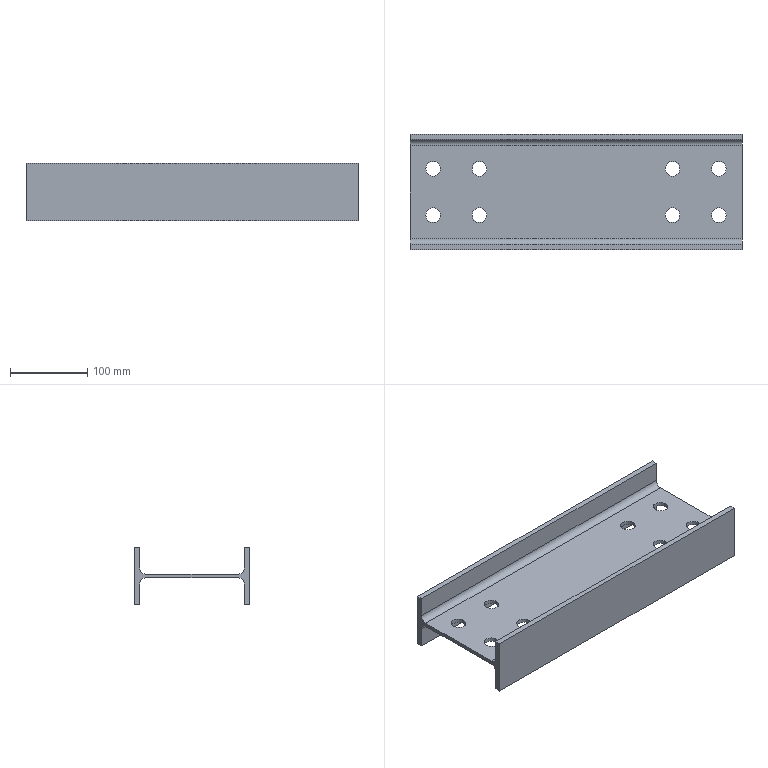Part | STEP file | 粉仓辅梁12_Default<As Machined> | 1 solid | 34 faces | box 430 x 150 x 75 mm | volume 756182 mm3 | cylinder 20 | plane 14 | commonest cylinder face diameters 19 x16 16 x4